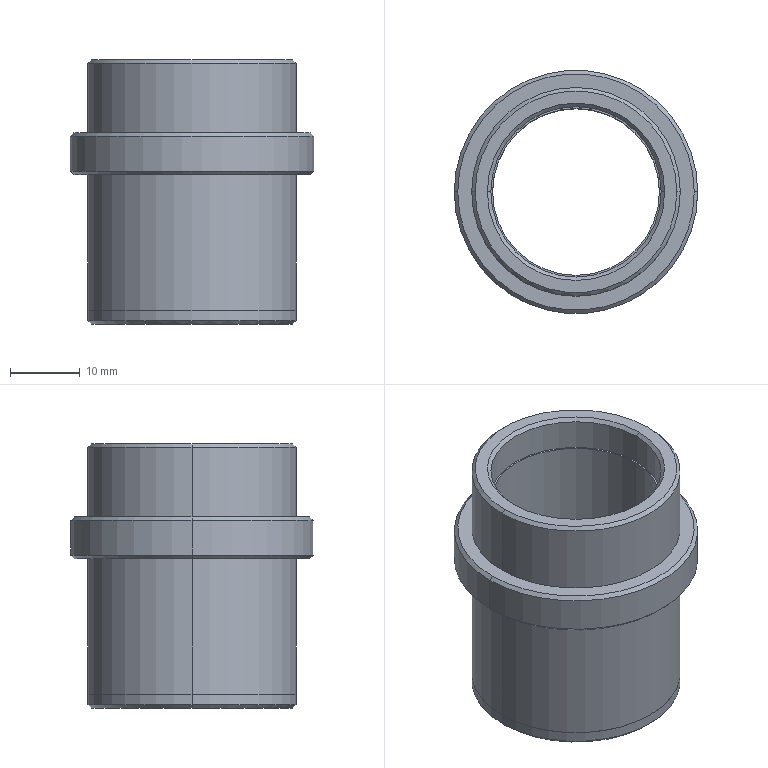Part | STEP file | Bucha inferior BEX - BEX2439 | 1 solid | 29 faces | box 35 x 35 x 38 mm | volume 10938 mm3 | cylinder 12 | cone 10 | plane 5 | torus 2 | commonest cylinder face diameters 30 x4 24 x2 24.5 x2 29.98 x2 35 x2